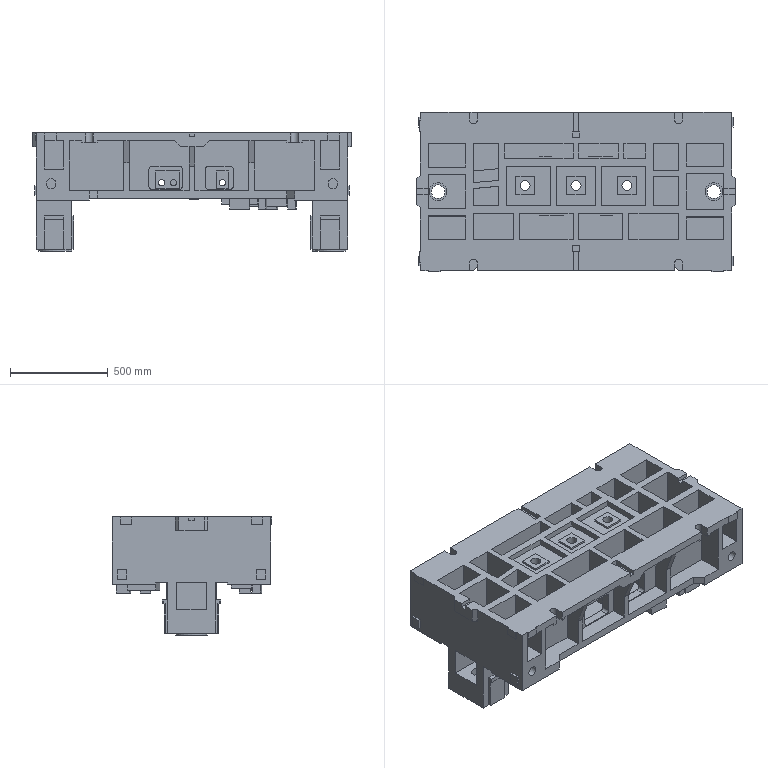Part | NX | features solid 2 | 1 solid | 568 faces | box 1630 x 815 x 605 mm | volume 209531072 mm3 | plane 507 | cylinder 60 | spline 1 | commonest cylinder face diameters 30 x22 80 x12 32 x6 40 x4 50 x4 10 x3